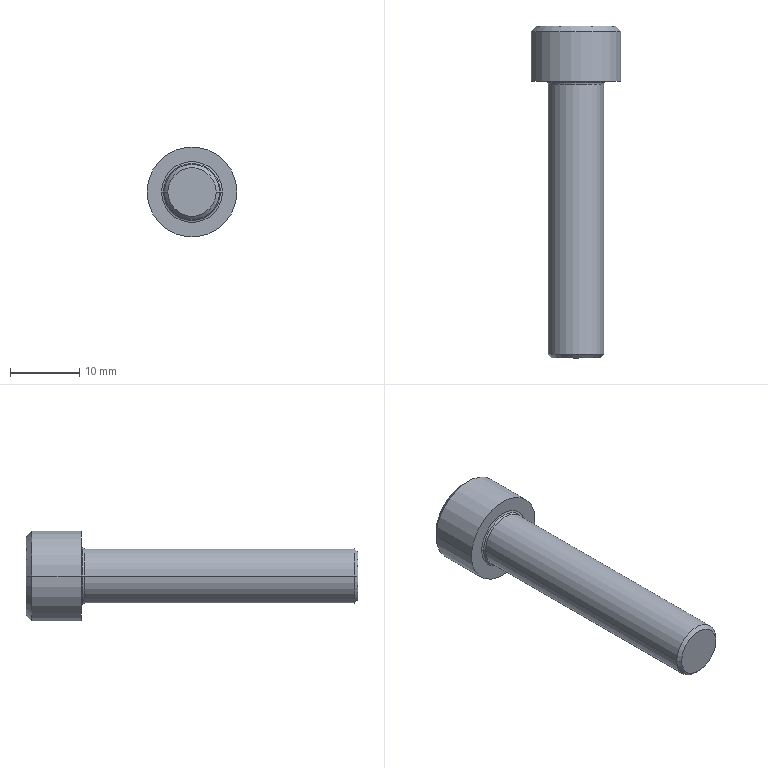Part | Creo | 1 solid | 23 faces | box 13 x 48 x 13 mm | volume 2909 mm3 | plane 9 | cone 6 | cylinder 4 | torus 4 | commonest cylinder face diameters 8 x2 13 x2
STEP:
#1=CARTESIAN_POINT('',(-76.536,361.995,-281.));
#2=VERTEX_POINT('',#1);
#3=CARTESIAN_POINT('',(-78.268,361.995,-284.));
#4=VERTEX_POINT('',#3);
#5=CARTESIAN_POINT('',(-76.536,361.995,-281.));
#6=CARTESIAN_POINT('',(-76.587,361.966,-281.088));
#7=CARTESIAN_POINT('',(-76.687,361.912,-281.261));
#8=CARTESIAN_POINT('',(-76.831,361.846,-281.511));
#9=CARTESIAN_POINT('',(-76.973,361.795,-281.757));
#10=CARTESIAN_POINT('',(-77.114,361.756,-282.002));
#11=CARTESIAN_POINT('',(-77.258,361.733,-282.25));
#12=CARTESIAN_POINT('',(-77.402,361.725,-282.5));
#13=CARTESIAN_POINT('',(-77.546,361.733,-282.75));
#14=CARTESIAN_POINT('',(-77.69,361.756,-282.998));
#15=CARTESIAN_POINT('',(-77.831,361.795,-283.243));
#16=CARTESIAN_POINT('',(-77.973,361.846,-283.489));
#17=CARTESIAN_POINT('',(-78.117,361.912,-283.739));
#18=CARTESIAN_POINT('',(-78.217,361.966,-283.912));
#19=CARTESIAN_POINT('',(-78.268,361.995,-284.));
#20=B_SPLINE_CURVE_WITH_KNOTS('',3,(#5,#6,#7,#8,#9,#10,#11,#12,#13,#14,#15,#16,#17,#18,#19),.UNSPECIFIED.,.F.,.F.,(4,1,1,1,1,1,1,1,1,1,1,1,4),(0.,0.08333,0.1667,0.25,0.3333,0.4167,0.5,0.5833,0.6667,0.75,0.8333,0.9167,1.),.UNSPECIFIED.);
#21=EDGE_CURVE('',#2,#4,#20,.T.);
#22=ORIENTED_EDGE('',*,*,#21,.F.);
#23=CARTESIAN_POINT('',(-80.,359.995,-281.));
#24=VERTEX_POINT('',#23);
#25=CARTESIAN_POINT('',(-80.,359.995,-281.));
#26=DIRECTION('',(0.866,0.5,0.));
#27=VECTOR('',#26,4.);
#28=LINE('',#25,#27);
#29=EDGE_CURVE('',#24,#2,#28,.T.);
#30=ORIENTED_EDGE('',*,*,#29,.F.);
#31=CARTESIAN_POINT('',(-83.464,361.995,-281.));
#32=VERTEX_POINT('',#31);
#33=CARTESIAN_POINT('',(-80.,359.995,-281.));
#34=DIRECTION('',(-0.866,0.5,0.));
#35=VECTOR('',#34,4.);
#36=LINE('',#33,#35);
#37=EDGE_CURVE('',#24,#32,#36,.T.);
#38=ORIENTED_EDGE('',*,*,#37,.T.);
#39=CARTESIAN_POINT('',(-81.732,361.995,-284.));
#40=VERTEX_POINT('',#39);
#41=CARTESIAN_POINT('',(-81.732,361.995,-284.));
#42=CARTESIAN_POINT('',(-81.783,361.966,-283.912));
#43=CARTESIAN_POINT('',(-81.883,361.912,-283.739));
#44=CARTESIAN_POINT('',(-82.027,361.846,-283.489));
#45=CARTESIAN_POINT('',(-82.169,361.795,-283.243));
#46=CARTESIAN_POINT('',(-82.31,361.756,-282.998));
#47=CARTESIAN_POINT('',(-82.454,361.733,-282.75));
#48=CARTESIAN_POINT('',(-82.598,361.725,-282.5));
#49=CARTESIAN_POINT('',(-82.742,361.733,-282.25));
#50=CARTESIAN_POINT('',(-82.886,361.756,-282.002));
#51=CARTESIAN_POINT('',(-83.027,361.795,-281.757));
#52=CARTESIAN_POINT('',(-83.169,361.846,-281.511));
#53=CARTESIAN_POINT('',(-83.313,361.912,-281.261));
#54=CARTESIAN_POINT('',(-83.413,361.966,-281.088));
#55=CARTESIAN_POINT('',(-83.464,361.995,-281.));
#56=B_SPLINE_CURVE_WITH_KNOTS('',3,(#41,#42,#43,#44,#45,#46,#47,#48,#49,#50,#51,#52,#53,#54,#55),.UNSPECIFIED.,.F.,.F.,(4,1,1,1,1,1,1,1,1,1,1,1,4),(0.,0.08333,0.1667,0.25,0.3333,0.4167,0.5,0.5833,0.6667,0.75,0.8333,0.9167,1.),.UNSPECIFIED.);
#57=EDGE_CURVE('',#40,#32,#56,.T.);
#58=ORIENTED_EDGE('',*,*,#57,.F.);
#59=CARTESIAN_POINT('',(-78.268,361.995,-284.));
#60=CARTESIAN_POINT('',(-78.369,361.966,-284.));
#61=CARTESIAN_POINT('',(-78.569,361.912,-284.));
#62=CARTESIAN_POINT('',(-78.857,361.847,-284.));
#63=CARTESIAN_POINT('',(-79.141,361.795,-284.));
#64=CARTESIAN_POINT('',(-79.424,361.757,-284.));
#65=CARTESIAN_POINT('',(-79.711,361.733,-284.));
#66=CARTESIAN_POINT('',(-80.,361.725,-284.));
#67=CARTESIAN_POINT('',(-80.289,361.733,-284.));
#68=CARTESIAN_POINT('',(-80.576,361.757,-284.));
#69=CARTESIAN_POINT('',(-80.859,361.795,-284.));
#70=CARTESIAN_POINT('',(-81.143,361.847,-284.));
#71=CARTESIAN_POINT('',(-81.431,361.912,-284.));
#72=CARTESIAN_POINT('',(-81.631,361.966,-284.));
#73=CARTESIAN_POINT('',(-81.732,361.995,-284.));
#74=B_SPLINE_CURVE_WITH_KNOTS('',3,(#59,#60,#61,#62,#63,#64,#65,#66,#67,#68,#69,#70,#71,#72,#73),.UNSPECIFIED.,.F.,.F.,(4,1,1,1,1,1,1,1,1,1,1,1,4),(0.,0.08333,0.1667,0.25,0.3333,0.4167,0.5,0.5833,0.6667,0.75,0.8333,0.9167,1.),.UNSPECIFIED.);
#75=EDGE_CURVE('',#4,#40,#74,.T.);
#76=ORIENTED_EDGE('',*,*,#75,.F.);
#77=EDGE_LOOP('',(#22,#30,#38,#58,#76));
#78=FACE_OUTER_BOUND('',#77,.F.);
#79=CARTESIAN_POINT('',(-80.,361.015,-281.));
#80=DIRECTION('',(0.,1.,0.));
#81=DIRECTION('',(1.,0.,0.));
#82=AXIS2_PLACEMENT_3D('',#79,#80,#81);
#83=CONICAL_SURFACE('',#82,1.767,60.);
#84=ADVANCED_FACE('',(#78),#83,.F.);
#85=CARTESIAN_POINT('',(-78.268,365.995,-284.));
#86=VERTEX_POINT('',#85);
#87=CARTESIAN_POINT('',(-76.536,365.995,-281.));
#88=VERTEX_POINT('',#87);
#89=CARTESIAN_POINT('',(-78.268,365.995,-284.));
#90=DIRECTION('',(0.5,0.,0.866));
#91=VECTOR('',#90,3.464);
#92=LINE('',#89,#91);
#93=EDGE_CURVE('',#86,#88,#92,.T.);
#94=ORIENTED_EDGE('',*,*,#93,.T.);
#95=CARTESIAN_POINT('',(-76.536,365.995,-281.));
#96=DIRECTION('',(0.,-1.,0.));
#97=VECTOR('',#96,4.);
#98=LINE('',#95,#97);
#99=EDGE_CURVE('',#88,#2,#98,.T.);
#100=ORIENTED_EDGE('',*,*,#99,.T.);
#101=ORIENTED_EDGE('',*,*,#21,.T.);
#102=CARTESIAN_POINT('',(-78.268,365.995,-284.));
#103=DIRECTION('',(0.,-1.,0.));
#104=VECTOR('',#103,4.);
#105=LINE('',#102,#104);
#106=EDGE_CURVE('',#86,#4,#105,.T.);
#107=ORIENTED_EDGE('',*,*,#106,.F.);
#108=EDGE_LOOP('',(#94,#100,#101,#107));
#109=FACE_OUTER_BOUND('',#108,.F.);
#110=CARTESIAN_POINT('',(-78.268,361.995,-284.));
#111=DIRECTION('',(-0.866,0.,0.5));
#112=DIRECTION('',(0.5,0.,0.866));
#113=AXIS2_PLACEMENT_3D('',#110,#111,#112);
#114=PLANE('',#113);
#115=ADVANCED_FACE('',(#109),#114,.T.);
#116=CARTESIAN_POINT('',(-74.3,365.995,-281.));
#117=VERTEX_POINT('',#116);
#118=CARTESIAN_POINT('',(-85.7,365.995,-281.));
#119=VERTEX_POINT('',#118);
#120=CARTESIAN_POINT('',(-80.,365.995,-281.));
#121=DIRECTION('',(0.,1.,0.));
#122=DIRECTION('',(1.,0.,0.));
#123=AXIS2_PLACEMENT_3D('',#120,#121,#122);
#124=CIRCLE('',#123,5.7);
#125=EDGE_CURVE('',#117,#119,#124,.T.);
#126=ORIENTED_EDGE('',*,*,#125,.F.);
#127=CARTESIAN_POINT('',(-80.,365.995,-281.));
#128=DIRECTION('',(0.,1.,0.));
#129=DIRECTION('',(-1.,0.,0.));
#130=AXIS2_PLACEMENT_3D('',#127,#128,#129);
#131=CIRCLE('',#130,5.7);
#132=EDGE_CURVE('',#119,#117,#131,.T.);
#133=ORIENTED_EDGE('',*,*,#132,.F.);
#134=EDGE_LOOP('',(#126,#133));
#135=FACE_OUTER_BOUND('',#134,.F.);
#136=CARTESIAN_POINT('',(-78.268,365.995,-278.));
#137=VERTEX_POINT('',#136);
#138=CARTESIAN_POINT('',(-76.536,365.995,-281.));
#139=DIRECTION('',(-0.5,0.,0.866));
#140=VECTOR('',#139,3.464);
#141=LINE('',#138,#140);
#142=EDGE_CURVE('',#88,#137,#141,.T.);
#143=ORIENTED_EDGE('',*,*,#142,.F.);
#144=ORIENTED_EDGE('',*,*,#93,.F.);
#145=CARTESIAN_POINT('',(-81.732,365.995,-284.));
#146=VERTEX_POINT('',#145);
#147=CARTESIAN_POINT('',(-78.268,365.995,-284.));
#148=DIRECTION('',(-1.,0.,0.));
#149=VECTOR('',#148,3.464);
#150=LINE('',#147,#149);
#151=EDGE_CURVE('',#86,#146,#150,.T.);
#152=ORIENTED_EDGE('',*,*,#151,.T.);
#153=CARTESIAN_POINT('',(-83.464,365.995,-281.));
#154=VERTEX_POINT('',#153);
#155=CARTESIAN_POINT('',(-83.464,365.995,-281.));
#156=DIRECTION('',(0.5,0.,-0.866));
#157=VECTOR('',#156,3.464);
#158=LINE('',#155,#157);
#159=EDGE_CURVE('',#154,#146,#158,.T.);
#160=ORIENTED_EDGE('',*,*,#159,.F.);
#161=CARTESIAN_POINT('',(-81.732,365.995,-278.));
#162=VERTEX_POINT('',#161);
#163=CARTESIAN_POINT('',(-81.732,365.995,-278.));
#164=DIRECTION('',(-0.5,0.,-0.866));
#165=VECTOR('',#164,3.464);
#166=LINE('',#163,#165);
#167=EDGE_CURVE('',#162,#154,#166,.T.);
#168=ORIENTED_EDGE('',*,*,#167,.F.);
#169=CARTESIAN_POINT('',(-81.732,365.995,-278.));
#170=DIRECTION('',(1.,0.,0.));
#171=VECTOR('',#170,3.464);
#172=LINE('',#169,#171);
#173=EDGE_CURVE('',#162,#137,#172,.T.);
#174=ORIENTED_EDGE('',*,*,#173,.T.);
#175=EDGE_LOOP('',(#143,#144,#152,#160,#168,#174));
#176=FACE_BOUND('',#175,.F.);
#177=CARTESIAN_POINT('',(-80.,365.995,-281.));
#178=DIRECTION('',(0.,1.,0.));
#179=DIRECTION('',(1.,0.,0.));
#180=AXIS2_PLACEMENT_3D('',#177,#178,#179);
#181=PLANE('',#180);
#182=ADVANCED_FACE('',(#135,#176),#181,.T.);
#183=CARTESIAN_POINT('',(-73.5,365.195,-281.));
#184=VERTEX_POINT('',#183);
#185=CARTESIAN_POINT('',(-86.5,365.195,-281.));
#186=VERTEX_POINT('',#185);
#187=CARTESIAN_POINT('',(-80.,365.195,-281.));
#188=DIRECTION('',(0.,1.,0.));
#189=DIRECTION('',(1.,0.,0.));
#190=AXIS2_PLACEMENT_3D('',#187,#188,#189);
#191=CIRCLE('',#190,6.5);
#192=EDGE_CURVE('',#184,#186,#191,.T.);
#193=ORIENTED_EDGE('',*,*,#192,.F.);
#194=CARTESIAN_POINT('',(-74.3,365.995,-281.));
#195=DIRECTION('',(0.7071,-0.7071,0.));
#196=VECTOR('',#195,1.131);
#197=LINE('',#194,#196);
#198=EDGE_CURVE('',#117,#184,#197,.T.);
#199=ORIENTED_EDGE('',*,*,#198,.F.);
#200=ORIENTED_EDGE('',*,*,#125,.T.);
#201=CARTESIAN_POINT('',(-85.7,365.995,-281.));
#202=DIRECTION('',(-0.7071,-0.7071,0.));
#203=VECTOR('',#202,1.131);
#204=LINE('',#201,#203);
#205=EDGE_CURVE('',#119,#186,#204,.T.);
#206=ORIENTED_EDGE('',*,*,#205,.T.);
#207=EDGE_LOOP('',(#193,#199,#200,#206));
#208=FACE_OUTER_BOUND('',#207,.F.);
#209=CARTESIAN_POINT('',(-80.,365.595,-281.));
#210=DIRECTION('',(0.,-1.,0.));
#211=DIRECTION('',(-1.,0.,0.));
#212=AXIS2_PLACEMENT_3D('',#209,#210,#211);
#213=CONICAL_SURFACE('',#212,6.1,45.);
#214=ADVANCED_FACE('',(#208),#213,.T.);
#215=ORIENTED_EDGE('',*,*,#192,.T.);
#216=CARTESIAN_POINT('',(-86.5,357.995,-281.));
#217=VERTEX_POINT('',#216);
#218=CARTESIAN_POINT('',(-86.5,357.995,-281.));
#219=DIRECTION('',(0.,1.,0.));
#220=VECTOR('',#219,7.2);
#221=LINE('',#218,#220);
#222=EDGE_CURVE('',#217,#186,#221,.T.);
#223=ORIENTED_EDGE('',*,*,#222,.F.);
#224=CARTESIAN_POINT('',(-73.5,357.995,-281.));
#225=VERTEX_POINT('',#224);
#226=CARTESIAN_POINT('',(-80.,357.995,-281.));
#227=DIRECTION('',(0.,-1.,0.));
#228=DIRECTION('',(-1.,0.,0.));
#229=AXIS2_PLACEMENT_3D('',#226,#227,#228);
#230=CIRCLE('',#229,6.5);
#231=EDGE_CURVE('',#217,#225,#230,.T.);
#232=ORIENTED_EDGE('',*,*,#231,.T.);
#233=CARTESIAN_POINT('',(-73.5,357.995,-281.));
#234=DIRECTION('',(0.,1.,0.));
#235=VECTOR('',#234,7.2);
#236=LINE('',#233,#235);
#237=EDGE_CURVE('',#225,#184,#236,.T.);
#238=ORIENTED_EDGE('',*,*,#237,.T.);
#239=EDGE_LOOP('',(#215,#223,#232,#238));
#240=FACE_OUTER_BOUND('',#239,.F.);
#241=CARTESIAN_POINT('',(-80.,357.995,-281.));
#242=DIRECTION('',(0.,1.,0.));
#243=DIRECTION('',(1.,0.,0.));
#244=AXIS2_PLACEMENT_3D('',#241,#242,#243);
#245=CYLINDRICAL_SURFACE('',#244,6.5);
#246=ADVANCED_FACE('',(#240),#245,.T.);
#247=CARTESIAN_POINT('',(-80.,365.195,-281.));
#248=DIRECTION('',(0.,1.,0.));
#249=DIRECTION('',(-1.,0.,0.));
#250=AXIS2_PLACEMENT_3D('',#247,#248,#249);
#251=CIRCLE('',#250,6.5);
#252=EDGE_CURVE('',#186,#184,#251,.T.);
#253=ORIENTED_EDGE('',*,*,#252,.T.);
#254=ORIENTED_EDGE('',*,*,#237,.F.);
#255=CARTESIAN_POINT('',(-80.,357.995,-281.));
#256=DIRECTION('',(0.,-1.,0.));
#257=DIRECTION('',(1.,0.,0.));
#258=AXIS2_PLACEMENT_3D('',#255,#256,#257);
#259=CIRCLE('',#258,6.5);
#260=EDGE_CURVE('',#225,#217,#259,.T.);
#261=ORIENTED_EDGE('',*,*,#260,.T.);
#262=ORIENTED_EDGE('',*,*,#222,.T.);
#263=EDGE_LOOP('',(#253,#254,#261,#262));
#264=FACE_OUTER_BOUND('',#263,.F.);
#265=CARTESIAN_POINT('',(-80.,357.995,-281.));
#266=DIRECTION('',(0.,1.,0.));
#267=DIRECTION('',(1.,0.,0.));
#268=AXIS2_PLACEMENT_3D('',#265,#266,#267);
#269=CYLINDRICAL_SURFACE('',#268,6.5);
#270=ADVANCED_FACE('',(#264),#269,.T.);
#271=ORIENTED_EDGE('',*,*,#252,.F.);
#272=ORIENTED_EDGE('',*,*,#205,.F.);
#273=ORIENTED_EDGE('',*,*,#132,.T.);
#274=ORIENTED_EDGE('',*,*,#198,.T.);
#275=EDGE_LOOP('',(#271,#272,#273,#274));
#276=FACE_OUTER_BOUND('',#275,.F.);
#277=CARTESIAN_POINT('',(-80.,365.595,-281.));
#278=DIRECTION('',(0.,-1.,0.));
#279=DIRECTION('',(-1.,0.,0.));
#280=AXIS2_PLACEMENT_3D('',#277,#278,#279);
#281=CONICAL_SURFACE('',#280,6.1,45.);
#282=ADVANCED_FACE('',(#276),#281,.T.);
#283=ORIENTED_EDGE('',*,*,#260,.F.);
#284=ORIENTED_EDGE('',*,*,#231,.F.);
#285=EDGE_LOOP('',(#283,#284));
#286=FACE_OUTER_BOUND('',#285,.F.);
#287=CARTESIAN_POINT('',(-75.6,357.995,-281.));
#288=VERTEX_POINT('',#287);
#289=CARTESIAN_POINT('',(-84.4,357.995,-281.));
#290=VERTEX_POINT('',#289);
#291=CARTESIAN_POINT('',(-80.,357.995,-281.));
#292=DIRECTION('',(0.,1.,0.));
#293=DIRECTION('',(1.,0.,0.));
#294=AXIS2_PLACEMENT_3D('',#291,#292,#293);
#295=CIRCLE('',#294,4.4);
#296=EDGE_CURVE('',#288,#290,#295,.T.);
#297=ORIENTED_EDGE('',*,*,#296,.F.);
#298=CARTESIAN_POINT('',(-80.,357.995,-281.));
#299=DIRECTION('',(0.,1.,0.));
#300=DIRECTION('',(-1.,0.,0.));
#301=AXIS2_PLACEMENT_3D('',#298,#299,#300);
#302=CIRCLE('',#301,4.4);
#303=EDGE_CURVE('',#290,#288,#302,.T.);
#304=ORIENTED_EDGE('',*,*,#303,.F.);
#305=EDGE_LOOP('',(#297,#304));
#306=FACE_BOUND('',#305,.F.);
#307=CARTESIAN_POINT('',(-80.,357.995,-281.));
#308=DIRECTION('',(0.,1.,0.));
#309=DIRECTION('',(1.,0.,0.));
#310=AXIS2_PLACEMENT_3D('',#307,#308,#309);
#311=PLANE('',#310);
#312=ADVANCED_FACE('',(#286,#306),#311,.F.);
#313=ORIENTED_EDGE('',*,*,#296,.T.);
#314=CARTESIAN_POINT('',(-84.117,357.878,-281.));
#315=VERTEX_POINT('',#314);
#316=CARTESIAN_POINT('',(-84.4,357.595,-281.));
#317=DIRECTION('',(0.,0.,-1.));
#318=DIRECTION('',(0.,1.,0.));
#319=AXIS2_PLACEMENT_3D('',#316,#317,#318);
#320=CIRCLE('',#319,0.4);
#321=EDGE_CURVE('',#290,#315,#320,.T.);
#322=ORIENTED_EDGE('',*,*,#321,.T.);
#323=CARTESIAN_POINT('',(-75.883,357.878,-281.));
#324=VERTEX_POINT('',#323);
#325=CARTESIAN_POINT('',(-80.,357.878,-281.));
#326=DIRECTION('',(0.,1.,0.));
#327=DIRECTION('',(1.,0.,0.));
#328=AXIS2_PLACEMENT_3D('',#325,#326,#327);
#329=CIRCLE('',#328,4.117);
#330=EDGE_CURVE('',#324,#315,#329,.T.);
#331=ORIENTED_EDGE('',*,*,#330,.F.);
#332=CARTESIAN_POINT('',(-75.6,357.595,-281.));
#333=DIRECTION('',(0.,0.,1.));
#334=DIRECTION('',(0.,1.,0.));
#335=AXIS2_PLACEMENT_3D('',#332,#333,#334);
#336=CIRCLE('',#335,0.4);
#337=EDGE_CURVE('',#288,#324,#336,.T.);
#338=ORIENTED_EDGE('',*,*,#337,.F.);
#339=EDGE_LOOP('',(#313,#322,#331,#338));
#340=FACE_OUTER_BOUND('',#339,.F.);
#341=CARTESIAN_POINT('',(-80.,357.595,-281.));
#342=DIRECTION('',(0.,1.,0.));
#343=DIRECTION('',(1.,0.,0.));
#344=AXIS2_PLACEMENT_3D('',#341,#342,#343);
#345=TOROIDAL_SURFACE('',#344,4.4,0.4);
#346=ADVANCED_FACE('',(#340),#345,.F.);
#347=ORIENTED_EDGE('',*,*,#303,.T.);
#348=ORIENTED_EDGE('',*,*,#337,.T.);
#349=CARTESIAN_POINT('',(-80.,357.878,-281.));
#350=DIRECTION('',(0.,1.,0.));
#351=DIRECTION('',(-1.,0.,0.));
#352=AXIS2_PLACEMENT_3D('',#349,#350,#351);
#353=CIRCLE('',#352,4.117);
#354=EDGE_CURVE('',#315,#324,#353,.T.);
#355=ORIENTED_EDGE('',*,*,#354,.F.);
#356=ORIENTED_EDGE('',*,*,#321,.F.);
#357=EDGE_LOOP('',(#347,#348,#355,#356));
#358=FACE_OUTER_BOUND('',#357,.F.);
#359=CARTESIAN_POINT('',(-80.,357.595,-281.));
#360=DIRECTION('',(0.,1.,0.));
#361=DIRECTION('',(1.,0.,0.));
#362=AXIS2_PLACEMENT_3D('',#359,#360,#361);
#363=TOROIDAL_SURFACE('',#362,4.4,0.4);
#364=ADVANCED_FACE('',(#358),#363,.F.);
#365=CARTESIAN_POINT('',(-84.,357.595,-281.));
#366=VERTEX_POINT('',#365);
#367=CARTESIAN_POINT('',(-76.,357.595,-281.));
#368=VERTEX_POINT('',#367);
#369=CARTESIAN_POINT('',(-80.,357.595,-281.));
#370=DIRECTION('',(0.,1.,0.));
#371=DIRECTION('',(-1.,0.,0.));
#372=AXIS2_PLACEMENT_3D('',#369,#370,#371);
#373=CIRCLE('',#372,4.);
#374=EDGE_CURVE('',#366,#368,#373,.T.);
#375=ORIENTED_EDGE('',*,*,#374,.F.);
#376=CARTESIAN_POINT('',(-84.4,357.595,-281.));
#377=DIRECTION('',(0.,0.,-1.));
#378=DIRECTION('',(0.7071,0.7071,0.));
#379=AXIS2_PLACEMENT_3D('',#376,#377,#378);
#380=CIRCLE('',#379,0.4);
#381=EDGE_CURVE('',#315,#366,#380,.T.);
#382=ORIENTED_EDGE('',*,*,#381,.F.);
#383=ORIENTED_EDGE('',*,*,#354,.T.);
#384=CARTESIAN_POINT('',(-75.6,357.595,-281.));
#385=DIRECTION('',(0.,0.,1.));
#386=DIRECTION('',(-0.7071,0.7071,0.));
#387=AXIS2_PLACEMENT_3D('',#384,#385,#386);
#388=CIRCLE('',#387,0.4);
#389=EDGE_CURVE('',#324,#368,#388,.T.);
#390=ORIENTED_EDGE('',*,*,#389,.T.);
#391=EDGE_LOOP('',(#375,#382,#383,#390));
#392=FACE_OUTER_BOUND('',#391,.F.);
#393=CARTESIAN_POINT('',(-80.,357.595,-281.));
#394=DIRECTION('',(0.,1.,0.));
#395=DIRECTION('',(1.,0.,0.));
#396=AXIS2_PLACEMENT_3D('',#393,#394,#395);
#397=TOROIDAL_SURFACE('',#396,4.4,0.4);
#398=ADVANCED_FACE('',(#392),#397,.F.);
#399=CARTESIAN_POINT('',(-76.,318.495,-281.));
#400=VERTEX_POINT('',#399);
#401=CARTESIAN_POINT('',(-84.,318.495,-281.));
#402=VERTEX_POINT('',#401);
#403=CARTESIAN_POINT('',(-80.,318.495,-281.));
#404=DIRECTION('',(0.,-1.,0.));
#405=DIRECTION('',(1.,0.,0.));
#406=AXIS2_PLACEMENT_3D('',#403,#404,#405);
#407=CIRCLE('',#406,4.);
#408=EDGE_CURVE('',#400,#402,#407,.T.);
#409=ORIENTED_EDGE('',*,*,#408,.T.);
#410=CARTESIAN_POINT('',(-84.,318.495,-281.));
#411=DIRECTION('',(0.,1.,0.));
#412=VECTOR('',#411,39.1);
#413=LINE('',#410,#412);
#414=EDGE_CURVE('',#402,#366,#413,.T.);
#415=ORIENTED_EDGE('',*,*,#414,.T.);
#416=ORIENTED_EDGE('',*,*,#374,.T.);
#417=CARTESIAN_POINT('',(-76.,318.495,-281.));
#418=DIRECTION('',(0.,1.,0.));
#419=VECTOR('',#418,39.1);
#420=LINE('',#417,#419);
#421=EDGE_CURVE('',#400,#368,#420,.T.);
#422=ORIENTED_EDGE('',*,*,#421,.F.);
#423=EDGE_LOOP('',(#409,#415,#416,#422));
#424=FACE_OUTER_BOUND('',#423,.F.);
#425=CARTESIAN_POINT('',(-80.,317.995,-281.));
#426=DIRECTION('',(0.,1.,0.));
#427=DIRECTION('',(1.,0.,0.));
#428=AXIS2_PLACEMENT_3D('',#425,#426,#427);
#429=CYLINDRICAL_SURFACE('',#428,4.);
#430=ADVANCED_FACE('',(#424),#429,.T.);
#431=CARTESIAN_POINT('',(-76.5,317.995,-281.));
#432=VERTEX_POINT('',#431);
#433=CARTESIAN_POINT('',(-83.5,317.995,-281.));
#434=VERTEX_POINT('',#433);
#435=CARTESIAN_POINT('',(-80.,317.995,-281.));
#436=DIRECTION('',(0.,-1.,0.));
#437=DIRECTION('',(1.,0.,0.));
#438=AXIS2_PLACEMENT_3D('',#435,#436,#437);
#439=CIRCLE('',#438,3.5);
#440=EDGE_CURVE('',#432,#434,#439,.T.);
#441=ORIENTED_EDGE('',*,*,#440,.T.);
#442=CARTESIAN_POINT('',(-83.5,317.995,-281.));
#443=DIRECTION('',(-0.7071,0.7071,0.));
#444=VECTOR('',#443,0.7071);
#445=LINE('',#442,#444);
#446=EDGE_CURVE('',#434,#402,#445,.T.);
#447=ORIENTED_EDGE('',*,*,#446,.T.);
#448=ORIENTED_EDGE('',*,*,#408,.F.);
#449=CARTESIAN_POINT('',(-76.5,317.995,-281.));
#450=DIRECTION('',(0.7071,0.7071,0.));
#451=VECTOR('',#450,0.7071);
#452=LINE('',#449,#451);
#453=EDGE_CURVE('',#432,#400,#452,.T.);
#454=ORIENTED_EDGE('',*,*,#453,.F.);
#455=EDGE_LOOP('',(#441,#447,#448,#454));
#456=FACE_OUTER_BOUND('',#455,.F.);
#457=CARTESIAN_POINT('',(-80.,318.245,-281.));
#458=DIRECTION('',(0.,1.,0.));
#459=DIRECTION('',(1.,0.,0.));
#460=AXIS2_PLACEMENT_3D('',#457,#458,#459);
#461=CONICAL_SURFACE('',#460,3.75,45.);
#462=ADVANCED_FACE('',(#456),#461,.T.);
#463=ORIENTED_EDGE('',*,*,#440,.F.);
#464=CARTESIAN_POINT('',(-80.,317.995,-281.));
#465=DIRECTION('',(0.,-1.,0.));
#466=DIRECTION('',(-1.,0.,0.));
#467=AXIS2_PLACEMENT_3D('',#464,#465,#466);
#468=CIRCLE('',#467,3.5);
#469=EDGE_CURVE('',#434,#432,#468,.T.);
#470=ORIENTED_EDGE('',*,*,#469,.F.);
#471=EDGE_LOOP('',(#463,#470));
#472=FACE_OUTER_BOUND('',#471,.F.);
#473=CARTESIAN_POINT('',(-80.,317.995,-281.));
#474=DIRECTION('',(0.,1.,0.));
#475=DIRECTION('',(1.,0.,0.));
#476=AXIS2_PLACEMENT_3D('',#473,#474,#475);
#477=PLANE('',#476);
#478=ADVANCED_FACE('',(#472),#477,.F.);
#479=ORIENTED_EDGE('',*,*,#469,.T.);
#480=ORIENTED_EDGE('',*,*,#453,.T.);
#481=CARTESIAN_POINT('',(-80.,318.495,-281.));
#482=DIRECTION('',(0.,-1.,0.));
#483=DIRECTION('',(-1.,0.,0.));
#484=AXIS2_PLACEMENT_3D('',#481,#482,#483);
#485=CIRCLE('',#484,4.);
#486=EDGE_CURVE('',#402,#400,#485,.T.);
#487=ORIENTED_EDGE('',*,*,#486,.F.);
#488=ORIENTED_EDGE('',*,*,#446,.F.);
#489=EDGE_LOOP('',(#479,#480,#487,#488));
#490=FACE_OUTER_BOUND('',#489,.F.);
#491=CARTESIAN_POINT('',(-80.,318.245,-281.));
#492=DIRECTION('',(0.,1.,0.));
#493=DIRECTION('',(1.,0.,0.));
#494=AXIS2_PLACEMENT_3D('',#491,#492,#493);
#495=CONICAL_SURFACE('',#494,3.75,45.);
#496=ADVANCED_FACE('',(#490),#495,.T.);
#497=ORIENTED_EDGE('',*,*,#486,.T.);
#498=ORIENTED_EDGE('',*,*,#421,.T.);
#499=CARTESIAN_POINT('',(-80.,357.595,-281.));
#500=DIRECTION('',(0.,1.,0.));
#501=DIRECTION('',(1.,0.,0.));
#502=AXIS2_PLACEMENT_3D('',#499,#500,#501);
#503=CIRCLE('',#502,4.);
#504=EDGE_CURVE('',#368,#366,#503,.T.);
#505=ORIENTED_EDGE('',*,*,#504,.T.);
#506=ORIENTED_EDGE('',*,*,#414,.F.);
#507=EDGE_LOOP('',(#497,#498,#505,#506));
#508=FACE_OUTER_BOUND('',#507,.F.);
#509=CARTESIAN_POINT('',(-80.,317.995,-281.));
#510=DIRECTION('',(0.,1.,0.));
#511=DIRECTION('',(1.,0.,0.));
#512=AXIS2_PLACEMENT_3D('',#509,#510,#511);
#513=CYLINDRICAL_SURFACE('',#512,4.);
#514=ADVANCED_FACE('',(#508),#513,.T.);
#515=ORIENTED_EDGE('',*,*,#504,.F.);
#516=ORIENTED_EDGE('',*,*,#389,.F.);
#517=ORIENTED_EDGE('',*,*,#330,.T.);
#518=ORIENTED_EDGE('',*,*,#381,.T.);
#519=EDGE_LOOP('',(#515,#516,#517,#518));
#520=FACE_OUTER_BOUND('',#519,.F.);
#521=CARTESIAN_POINT('',(-80.,357.595,-281.));
#522=DIRECTION('',(0.,1.,0.));
#523=DIRECTION('',(1.,0.,0.));
#524=AXIS2_PLACEMENT_3D('',#521,#522,#523);
#525=TOROIDAL_SURFACE('',#524,4.4,0.4);
#526=ADVANCED_FACE('',(#520),#525,.F.);
#527=ORIENTED_EDGE('',*,*,#142,.T.);
#528=CARTESIAN_POINT('',(-78.268,361.995,-278.));
#529=VERTEX_POINT('',#528);
#530=CARTESIAN_POINT('',(-78.268,365.995,-278.));
#531=DIRECTION('',(0.,-1.,0.));
#532=VECTOR('',#531,4.);
#533=LINE('',#530,#532);
#534=EDGE_CURVE('',#137,#529,#533,.T.);
#535=ORIENTED_EDGE('',*,*,#534,.T.);
#536=CARTESIAN_POINT('',(-78.268,361.995,-278.));
#537=CARTESIAN_POINT('',(-78.217,361.966,-278.088));
#538=CARTESIAN_POINT('',(-78.117,361.912,-278.261));
#539=CARTESIAN_POINT('',(-77.973,361.846,-278.511));
#540=CARTESIAN_POINT('',(-77.831,361.795,-278.757));
#541=CARTESIAN_POINT('',(-77.69,361.756,-279.002));
#542=CARTESIAN_POINT('',(-77.546,361.733,-279.25));
#543=CARTESIAN_POINT('',(-77.402,361.725,-279.5));
#544=CARTESIAN_POINT('',(-77.258,361.733,-279.75));
#545=CARTESIAN_POINT('',(-77.114,361.756,-279.998));
#546=CARTESIAN_POINT('',(-76.973,361.795,-280.243));
#547=CARTESIAN_POINT('',(-76.831,361.846,-280.489));
#548=CARTESIAN_POINT('',(-76.687,361.912,-280.739));
#549=CARTESIAN_POINT('',(-76.587,361.966,-280.912));
#550=CARTESIAN_POINT('',(-76.536,361.995,-281.));
#551=B_SPLINE_CURVE_WITH_KNOTS('',3,(#536,#537,#538,#539,#540,#541,#542,#543,#544,#545,#546,#547,#548,#549,#550),.UNSPECIFIED.,.F.,.F.,(4,1,1,1,1,1,1,1,1,1,1,1,4),(0.,0.08333,0.1667,0.25,0.3333,0.4167,0.5,0.5833,0.6667,0.75,0.8333,0.9167,1.),.UNSPECIFIED.);
#552=EDGE_CURVE('',#529,#2,#551,.T.);
#553=ORIENTED_EDGE('',*,*,#552,.T.);
#554=ORIENTED_EDGE('',*,*,#99,.F.);
#555=EDGE_LOOP('',(#527,#535,#553,#554));
#556=FACE_OUTER_BOUND('',#555,.F.);
#557=CARTESIAN_POINT('',(-76.536,361.995,-281.));
#558=DIRECTION('',(-0.866,0.,-0.5));
#559=DIRECTION('',(-0.5,0.,0.866));
#560=AXIS2_PLACEMENT_3D('',#557,#558,#559);
#561=PLANE('',#560);
#562=ADVANCED_FACE('',(#556),#561,.T.);
#563=ORIENTED_EDGE('',*,*,#173,.F.);
#564=CARTESIAN_POINT('',(-81.732,361.995,-278.));
#565=VERTEX_POINT('',#564);
#566=CARTESIAN_POINT('',(-81.732,365.995,-278.));
#567=DIRECTION('',(0.,-1.,0.));
#568=VECTOR('',#567,4.);
#569=LINE('',#566,#568);
#570=EDGE_CURVE('',#162,#565,#569,.T.);
#571=ORIENTED_EDGE('',*,*,#570,.T.);
#572=CARTESIAN_POINT('',(-81.732,361.995,-278.));
#573=CARTESIAN_POINT('',(-81.631,361.966,-278.));
#574=CARTESIAN_POINT('',(-81.431,361.912,-278.));
#575=CARTESIAN_POINT('',(-81.143,361.847,-278.));
#576=CARTESIAN_POINT('',(-80.859,361.795,-278.));
#577=CARTESIAN_POINT('',(-80.576,361.757,-278.));
#578=CARTESIAN_POINT('',(-80.289,361.733,-278.));
#579=CARTESIAN_POINT('',(-80.,361.725,-278.));
#580=CARTESIAN_POINT('',(-79.711,361.733,-278.));
#581=CARTESIAN_POINT('',(-79.424,361.757,-278.));
#582=CARTESIAN_POINT('',(-79.141,361.795,-278.));
#583=CARTESIAN_POINT('',(-78.857,361.847,-278.));
#584=CARTESIAN_POINT('',(-78.569,361.912,-278.));
#585=CARTESIAN_POINT('',(-78.369,361.966,-278.));
#586=CARTESIAN_POINT('',(-78.268,361.995,-278.));
#587=B_SPLINE_CURVE_WITH_KNOTS('',3,(#572,#573,#574,#575,#576,#577,#578,#579,#580,#581,#582,#583,#584,#585,#586),.UNSPECIFIED.,.F.,.F.,(4,1,1,1,1,1,1,1,1,1,1,1,4),(0.,0.08333,0.1667,0.25,0.3333,0.4167,0.5,0.5833,0.6667,0.75,0.8333,0.9167,1.),.UNSPECIFIED.);
#588=EDGE_CURVE('',#565,#529,#587,.T.);
#589=ORIENTED_EDGE('',*,*,#588,.T.);
#590=ORIENTED_EDGE('',*,*,#534,.F.);
#591=EDGE_LOOP('',(#563,#571,#589,#590));
#592=FACE_OUTER_BOUND('',#591,.F.);
#593=CARTESIAN_POINT('',(-78.268,361.995,-278.));
#594=DIRECTION('',(0.,0.,-1.));
#595=DIRECTION('',(0.,1.,0.));
#596=AXIS2_PLACEMENT_3D('',#593,#594,#595);
#597=PLANE('',#596);
#598=ADVANCED_FACE('',(#592),#597,.T.);
#599=ORIENTED_EDGE('',*,*,#167,.T.);
#600=CARTESIAN_POINT('',(-83.464,365.995,-281.));
#601=DIRECTION('',(0.,-1.,0.));
#602=VECTOR('',#601,4.);
#603=LINE('',#600,#602);
#604=EDGE_CURVE('',#154,#32,#603,.T.);
#605=ORIENTED_EDGE('',*,*,#604,.T.);
#606=CARTESIAN_POINT('',(-83.464,361.995,-281.));
#607=CARTESIAN_POINT('',(-83.413,361.966,-280.912));
#608=CARTESIAN_POINT('',(-83.313,361.912,-280.739));
#609=CARTESIAN_POINT('',(-83.169,361.846,-280.489));
#610=CARTESIAN_POINT('',(-83.027,361.795,-280.243));
#611=CARTESIAN_POINT('',(-82.886,361.756,-279.998));
#612=CARTESIAN_POINT('',(-82.742,361.733,-279.75));
#613=CARTESIAN_POINT('',(-82.598,361.725,-279.5));
#614=CARTESIAN_POINT('',(-82.454,361.733,-279.25));
#615=CARTESIAN_POINT('',(-82.31,361.756,-279.002));
#616=CARTESIAN_POINT('',(-82.169,361.795,-278.757));
#617=CARTESIAN_POINT('',(-82.027,361.846,-278.511));
#618=CARTESIAN_POINT('',(-81.883,361.912,-278.261));
#619=CARTESIAN_POINT('',(-81.783,361.966,-278.088));
#620=CARTESIAN_POINT('',(-81.732,361.995,-278.));
#621=B_SPLINE_CURVE_WITH_KNOTS('',3,(#606,#607,#608,#609,#610,#611,#612,#613,#614,#615,#616,#617,#618,#619,#620),.UNSPECIFIED.,.F.,.F.,(4,1,1,1,1,1,1,1,1,1,1,1,4),(0.,0.08333,0.1667,0.25,0.3333,0.4167,0.5,0.5833,0.6667,0.75,0.8333,0.9167,1.),.UNSPECIFIED.);
#622=EDGE_CURVE('',#32,#565,#621,.T.);
#623=ORIENTED_EDGE('',*,*,#622,.T.);
#624=ORIENTED_EDGE('',*,*,#570,.F.);
#625=EDGE_LOOP('',(#599,#605,#623,#624));
#626=FACE_OUTER_BOUND('',#625,.F.);
#627=CARTESIAN_POINT('',(-81.732,361.995,-278.));
#628=DIRECTION('',(0.866,0.,-0.5));
#629=DIRECTION('',(-0.5,0.,-0.866));
#630=AXIS2_PLACEMENT_3D('',#627,#628,#629);
#631=PLANE('',#630);
#632=ADVANCED_FACE('',(#626),#631,.T.);
#633=ORIENTED_EDGE('',*,*,#159,.T.);
#634=CARTESIAN_POINT('',(-81.732,365.995,-284.));
#635=DIRECTION('',(0.,-1.,0.));
#636=VECTOR('',#635,4.);
#637=LINE('',#634,#636);
#638=EDGE_CURVE('',#146,#40,#637,.T.);
#639=ORIENTED_EDGE('',*,*,#638,.T.);
#640=ORIENTED_EDGE('',*,*,#57,.T.);
#641=ORIENTED_EDGE('',*,*,#604,.F.);
#642=EDGE_LOOP('',(#633,#639,#640,#641));
#643=FACE_OUTER_BOUND('',#642,.F.);
#644=CARTESIAN_POINT('',(-83.464,361.995,-281.));
#645=DIRECTION('',(0.866,0.,0.5));
#646=DIRECTION('',(0.5,0.,-0.866));
#647=AXIS2_PLACEMENT_3D('',#644,#645,#646);
#648=PLANE('',#647);
#649=ADVANCED_FACE('',(#643),#648,.T.);
#650=ORIENTED_EDGE('',*,*,#151,.F.);
#651=ORIENTED_EDGE('',*,*,#106,.T.);
#652=ORIENTED_EDGE('',*,*,#75,.T.);
#653=ORIENTED_EDGE('',*,*,#638,.F.);
#654=EDGE_LOOP('',(#650,#651,#652,#653));
#655=FACE_OUTER_BOUND('',#654,.F.);
#656=CARTESIAN_POINT('',(-81.732,361.995,-284.));
#657=DIRECTION('',(0.,0.,1.));
#658=DIRECTION('',(0.,-1.,0.));
#659=AXIS2_PLACEMENT_3D('',#656,#657,#658);
#660=PLANE('',#659);
#661=ADVANCED_FACE('',(#655),#660,.T.);
#662=ORIENTED_EDGE('',*,*,#622,.F.);
#663=ORIENTED_EDGE('',*,*,#37,.F.);
#664=ORIENTED_EDGE('',*,*,#29,.T.);
#665=ORIENTED_EDGE('',*,*,#552,.F.);
#666=ORIENTED_EDGE('',*,*,#588,.F.);
#667=EDGE_LOOP('',(#662,#663,#664,#665,#666));
#668=FACE_OUTER_BOUND('',#667,.F.);
#669=CARTESIAN_POINT('',(-80.,361.015,-281.));
#670=DIRECTION('',(0.,1.,0.));
#671=DIRECTION('',(1.,0.,0.));
#672=AXIS2_PLACEMENT_3D('',#669,#670,#671);
#673=CONICAL_SURFACE('',#672,1.767,60.);
#674=ADVANCED_FACE('',(#668),#673,.F.);
#675=CLOSED_SHELL('',(#84,#115,#182,#214,#246,#270,#282,#312,#346,#364,#398,#430,#462,#478,#496,#514,#526,#562,#598,#632,#649,#661,#674));
#676=MANIFOLD_SOLID_BREP('',#675);
#677=(LENGTH_UNIT()NAMED_UNIT(*)SI_UNIT(.MILLI.,.METRE.));
#678=UNCERTAINTY_MEASURE_WITH_UNIT(LENGTH_MEASURE(0.00514),#677,'','');
#679=(NAMED_UNIT(*)PLANE_ANGLE_UNIT()SI_UNIT($,.RADIAN.));
#680=PLANE_ANGLE_MEASURE_WITH_UNIT(PLANE_ANGLE_MEASURE(0.01745),#679);
#681=(CONVERSION_BASED_UNIT('DEGREE',#680)NAMED_UNIT(*)PLANE_ANGLE_UNIT());
#682=(NAMED_UNIT(*)SI_UNIT($,.STERADIAN.)SOLID_ANGLE_UNIT());
#683=(GEOMETRIC_REPRESENTATION_CONTEXT(3)GLOBAL_UNCERTAINTY_ASSIGNED_CONTEXT((#678))GLOBAL_UNIT_ASSIGNED_CONTEXT((#677,#681,#682))REPRESENTATION_CONTEXT('',''));
#684=ADVANCED_BREP_SHAPE_REPRESENTATION('',(#676),#683);